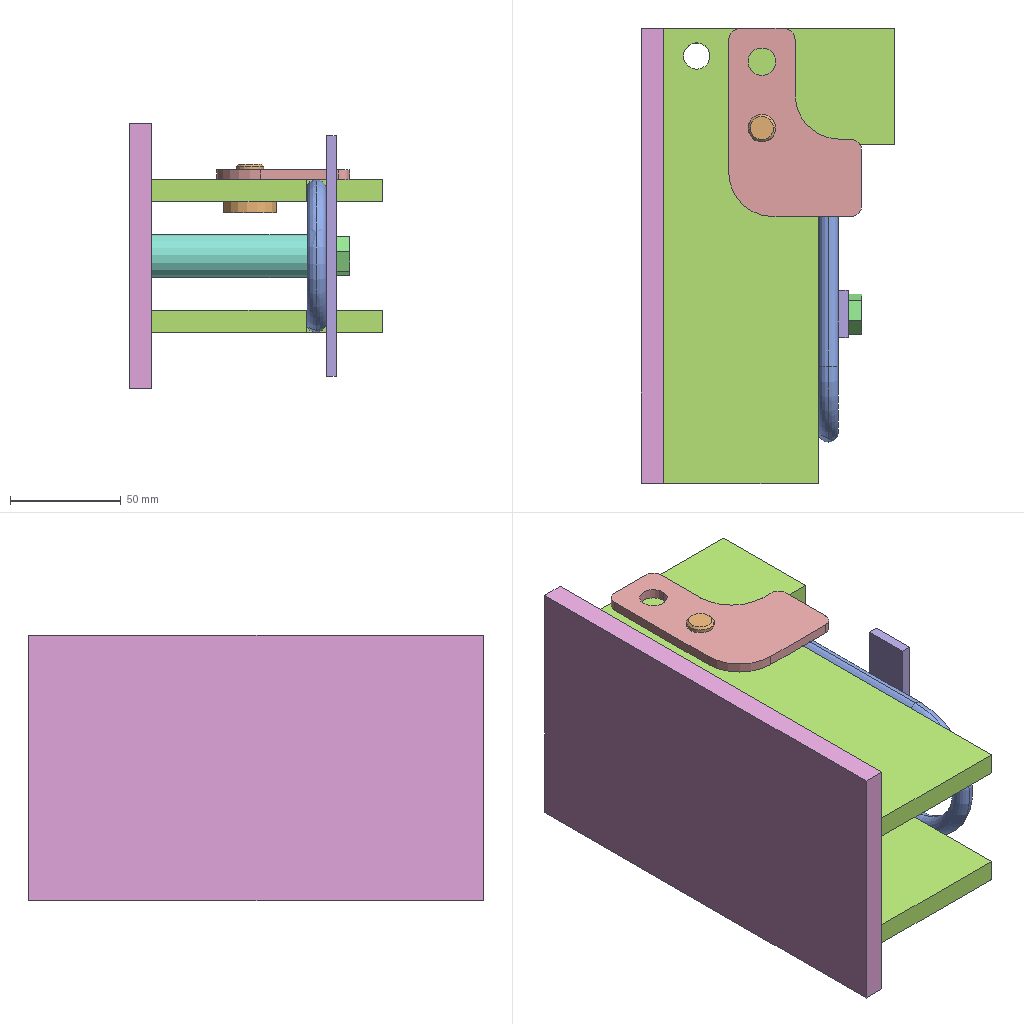Assembly | SolidWorks | 9 different items | 10 placed | box 115 x 205 x 120 mm
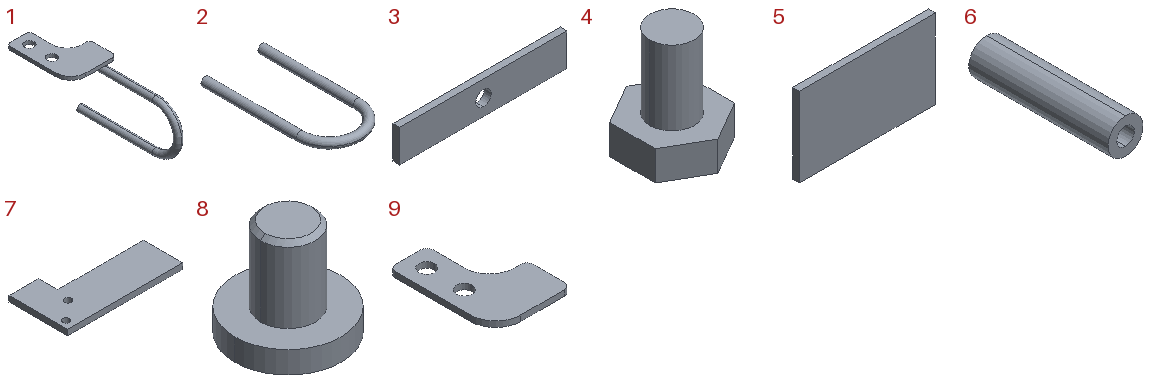Parts list (item | name | quantity | parent item | size | volume | features):
1 | (subassembly) | x1 | - | 60 x 186.95 x 73.5 mm | 33718 mm3 | features CompositeCurve 1
2 | - | x1 | in 1 | 69 x 134.5 x 9 mm | 18719 mm3 | features Sweep 1
3 | - | x1 | - | 108.732 x 4.5 x 21.168 mm | 10004 mm3 | features Extrusion 1
4 | - | x1 | - | 16 x 18.475 x 21 mm | 2284 mm3 | features Extrusion 1, ICE 1
5 | - | x1 | - | 205.392 x 10 x 120 mm | 246471 mm3 | features Extrusion 1
6 | - | x1 | - | 20 x 79 x 20 mm | 18614 mm3 | features Extrusion 1
7 | - | x2 | - | 205.392 x 104.5 x 10 mm | 159512 mm3 | features Extrusion 1
8 | - | x1 | - | 24.181 x 24.181 x 22 mm | 4364 mm3 | features Chamfer 1, Extrusion 1, ICE 1
9 | - | x1 | in 1 | 60 x 85 x 4.5 mm | 14999 mm3 | features Extrusion 1
Mates (type | each side: item.copy, entity, surface, feature):
In the top assembly
Coincident | 2.1 face plane Sweep1 | 7.1 face plane Boss-Extrude1
Coincident | 9.1 face plane Boss-Extrude1 | 7.1 face plane Boss-Extrude1
DistanceDim | 9.1 face plane Boss-Extrude1 | 7.1 face plane Boss-Extrude1
Coincident | 7.1 face plane Boss-Extrude1 | 7.2 face plane Boss-Extrude1 | 2 times
DistanceDim | 7.1 face plane Boss-Extrude1 | 7.2 face plane Boss-Extrude1
Coincident | 7.2 face plane Boss-Extrude1 | 5.1 face plane Boss-Extrude1
DistanceDim | 7.1 face plane Boss-Extrude1 | 5.1 face plane Boss-Extrude1
Coincident | 5.1 face plane Boss-Extrude1 | 6.1 face plane Boss-Extrude1
Coincident | 7.1 face plane Boss-Extrude1 | 5.1 face plane Boss-Extrude1
Coincident | 7.1 face plane Boss-Extrude1 | 8.1 edge
Concentric | 9.1 edge | 8.1 edge
Parallel | 7.2 face plane Boss-Extrude1 | 3.1 face plane Boss-Extrude1
Coincident | 6.1 face plane Boss-Extrude1 | 3.1 face plane Boss-Extrude1
Concentric | 6.1 edge | 3.1 edge
Concentric | 3.1 edge | 4.1 edge
Coincident | 3.1 face plane Boss-Extrude1 | 4.1 face plane Boss-Extrude2
In subassembly 1
DistanceDim | 9.2 face plane Boss-Extrude1 | 2.2 face plane Sweep1
Coincident | 1.1 face | 1.1 face | 4 times
Concentric | 9.2 edge | 1.1 edge
DistanceDim | 1.1 face | 1.1 face | 2 times
Concentric | 1.1 edge | 1.1 select_type:0
Coincident | 1.1 edge | 1.1 select_type:0 | 2 times